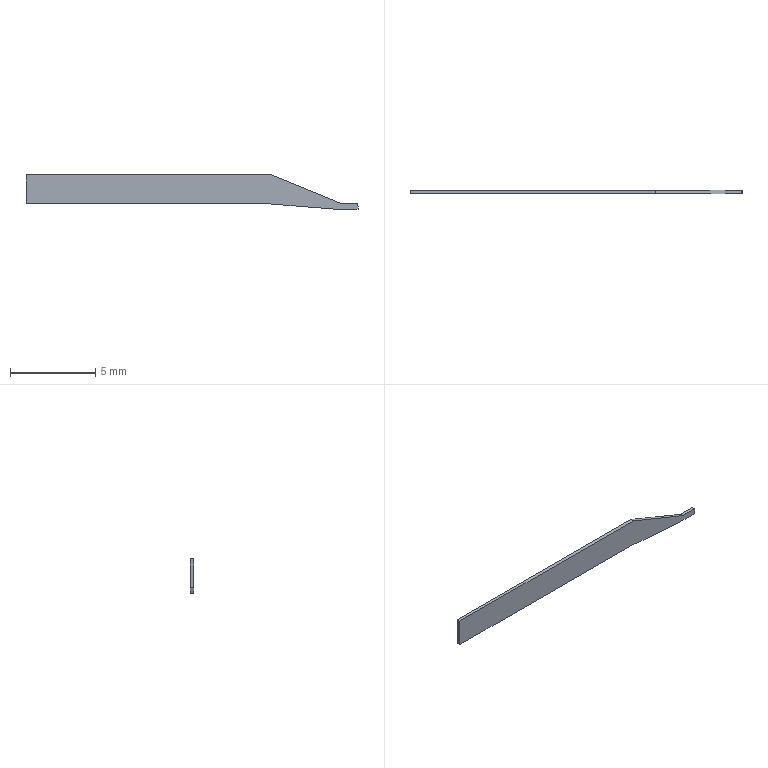Part | SolidWorks | features Extrusion 1 | 1 solid | 10 faces | box 19.5 x 0.2 x 2.02 mm | volume 5.825 mm3 | plane 10
STEP:
#1=CARTESIAN_POINT('',(0.,0.,-1.7));
#2=VERTEX_POINT('',#1);
#3=CARTESIAN_POINT('',(0.,0.,0.));
#4=VERTEX_POINT('',#3);
#5=CARTESIAN_POINT('',(0.,0.,0.));
#6=DIRECTION('',(0.,0.,1.));
#7=VECTOR('',#6,1000.);
#8=LINE('',#5,#7);
#9=EDGE_CURVE('',#2,#4,#8,.T.);
#10=ORIENTED_EDGE('',*,*,#9,.T.);
#11=CARTESIAN_POINT('',(0.,0.2,0.));
#12=VERTEX_POINT('',#11);
#13=CARTESIAN_POINT('',(0.,0.2,0.));
#14=DIRECTION('',(0.,-1.,0.));
#15=VECTOR('',#14,1000.);
#16=LINE('',#13,#15);
#17=EDGE_CURVE('',#12,#4,#16,.T.);
#18=ORIENTED_EDGE('',*,*,#17,.F.);
#19=CARTESIAN_POINT('',(0.,0.2,-1.7));
#20=VERTEX_POINT('',#19);
#21=CARTESIAN_POINT('',(0.,0.2,0.));
#22=DIRECTION('',(0.,0.,1.));
#23=VECTOR('',#22,1000.);
#24=LINE('',#21,#23);
#25=EDGE_CURVE('',#20,#12,#24,.T.);
#26=ORIENTED_EDGE('',*,*,#25,.F.);
#27=CARTESIAN_POINT('',(0.,0.2,-1.7));
#28=DIRECTION('',(0.,-1.,0.));
#29=VECTOR('',#28,1000.);
#30=LINE('',#27,#29);
#31=EDGE_CURVE('',#20,#2,#30,.T.);
#32=ORIENTED_EDGE('',*,*,#31,.T.);
#33=EDGE_LOOP('',(#10,#18,#26,#32));
#34=FACE_OUTER_BOUND('',#33,.T.);
#35=CARTESIAN_POINT('',(0.,0.2,0.));
#36=DIRECTION('',(1.,0.,0.));
#37=DIRECTION('',(0.,0.,-1.));
#38=AXIS2_PLACEMENT_3D('',#35,#36,#37);
#39=PLANE('',#38);
#40=ADVANCED_FACE('',(#34),#39,.F.);
#41=CARTESIAN_POINT('',(14.408,0.,0.));
#42=VERTEX_POINT('',#41);
#43=CARTESIAN_POINT('',(0.,0.,0.));
#44=DIRECTION('',(1.,0.,0.));
#45=VECTOR('',#44,1000.);
#46=LINE('',#43,#45);
#47=EDGE_CURVE('',#4,#42,#46,.T.);
#48=ORIENTED_EDGE('',*,*,#47,.T.);
#49=CARTESIAN_POINT('',(14.408,0.2,0.));
#50=VERTEX_POINT('',#49);
#51=CARTESIAN_POINT('',(14.408,0.2,0.));
#52=DIRECTION('',(0.,-1.,0.));
#53=VECTOR('',#52,1000.);
#54=LINE('',#51,#53);
#55=EDGE_CURVE('',#50,#42,#54,.T.);
#56=ORIENTED_EDGE('',*,*,#55,.F.);
#57=CARTESIAN_POINT('',(0.,0.2,0.));
#58=DIRECTION('',(1.,0.,0.));
#59=VECTOR('',#58,1000.);
#60=LINE('',#57,#59);
#61=EDGE_CURVE('',#12,#50,#60,.T.);
#62=ORIENTED_EDGE('',*,*,#61,.F.);
#63=ORIENTED_EDGE('',*,*,#17,.T.);
#64=EDGE_LOOP('',(#48,#56,#62,#63));
#65=FACE_OUTER_BOUND('',#64,.T.);
#66=CARTESIAN_POINT('',(0.,0.2,0.));
#67=DIRECTION('',(0.,0.,-1.));
#68=DIRECTION('',(-1.,0.,0.));
#69=AXIS2_PLACEMENT_3D('',#66,#67,#68);
#70=PLANE('',#69);
#71=ADVANCED_FACE('',(#65),#70,.F.);
#72=CARTESIAN_POINT('',(18.5,0.,-1.67));
#73=VERTEX_POINT('',#72);
#74=CARTESIAN_POINT('',(18.5,0.,-1.67));
#75=DIRECTION('',(0.9259,0.,-0.3778));
#76=VECTOR('',#75,1000.);
#77=LINE('',#74,#76);
#78=EDGE_CURVE('',#42,#73,#77,.T.);
#79=ORIENTED_EDGE('',*,*,#78,.T.);
#80=CARTESIAN_POINT('',(18.5,0.2,-1.67));
#81=VERTEX_POINT('',#80);
#82=CARTESIAN_POINT('',(18.5,0.2,-1.67));
#83=DIRECTION('',(0.,-1.,0.));
#84=VECTOR('',#83,1000.);
#85=LINE('',#82,#84);
#86=EDGE_CURVE('',#81,#73,#85,.T.);
#87=ORIENTED_EDGE('',*,*,#86,.F.);
#88=CARTESIAN_POINT('',(18.5,0.2,-1.67));
#89=DIRECTION('',(0.9259,0.,-0.3778));
#90=VECTOR('',#89,1000.);
#91=LINE('',#88,#90);
#92=EDGE_CURVE('',#50,#81,#91,.T.);
#93=ORIENTED_EDGE('',*,*,#92,.F.);
#94=ORIENTED_EDGE('',*,*,#55,.T.);
#95=EDGE_LOOP('',(#79,#87,#93,#94));
#96=FACE_OUTER_BOUND('',#95,.T.);
#97=CARTESIAN_POINT('',(18.5,0.2,-1.67));
#98=DIRECTION('',(-0.3778,0.,-0.9259));
#99=DIRECTION('',(-0.9259,0.,0.3778));
#100=AXIS2_PLACEMENT_3D('',#97,#98,#99);
#101=PLANE('',#100);
#102=ADVANCED_FACE('',(#96),#101,.F.);
#103=CARTESIAN_POINT('',(19.5,0.,-1.67));
#104=VERTEX_POINT('',#103);
#105=CARTESIAN_POINT('',(19.5,0.,-1.67));
#106=DIRECTION('',(1.,0.,0.));
#107=VECTOR('',#106,1000.);
#108=LINE('',#105,#107);
#109=EDGE_CURVE('',#73,#104,#108,.T.);
#110=ORIENTED_EDGE('',*,*,#109,.T.);
#111=CARTESIAN_POINT('',(19.5,0.2,-1.67));
#112=VERTEX_POINT('',#111);
#113=CARTESIAN_POINT('',(19.5,0.2,-1.67));
#114=DIRECTION('',(0.,-1.,0.));
#115=VECTOR('',#114,1000.);
#116=LINE('',#113,#115);
#117=EDGE_CURVE('',#112,#104,#116,.T.);
#118=ORIENTED_EDGE('',*,*,#117,.F.);
#119=CARTESIAN_POINT('',(19.5,0.2,-1.67));
#120=DIRECTION('',(1.,0.,0.));
#121=VECTOR('',#120,1000.);
#122=LINE('',#119,#121);
#123=EDGE_CURVE('',#81,#112,#122,.T.);
#124=ORIENTED_EDGE('',*,*,#123,.F.);
#125=ORIENTED_EDGE('',*,*,#86,.T.);
#126=EDGE_LOOP('',(#110,#118,#124,#125));
#127=FACE_OUTER_BOUND('',#126,.T.);
#128=CARTESIAN_POINT('',(19.5,0.2,-1.67));
#129=DIRECTION('',(0.,0.,-1.));
#130=DIRECTION('',(-1.,0.,0.));
#131=AXIS2_PLACEMENT_3D('',#128,#129,#130);
#132=PLANE('',#131);
#133=ADVANCED_FACE('',(#127),#132,.F.);
#134=CARTESIAN_POINT('',(19.5,0.,-2.02));
#135=VERTEX_POINT('',#134);
#136=CARTESIAN_POINT('',(19.5,0.,-1.67));
#137=DIRECTION('',(0.,0.,-1.));
#138=VECTOR('',#137,1000.);
#139=LINE('',#136,#138);
#140=EDGE_CURVE('',#104,#135,#139,.T.);
#141=ORIENTED_EDGE('',*,*,#140,.T.);
#142=CARTESIAN_POINT('',(19.5,0.2,-2.02));
#143=VERTEX_POINT('',#142);
#144=CARTESIAN_POINT('',(19.5,0.2,-2.02));
#145=DIRECTION('',(0.,-1.,0.));
#146=VECTOR('',#145,1000.);
#147=LINE('',#144,#146);
#148=EDGE_CURVE('',#143,#135,#147,.T.);
#149=ORIENTED_EDGE('',*,*,#148,.F.);
#150=CARTESIAN_POINT('',(19.5,0.2,-1.67));
#151=DIRECTION('',(0.,0.,-1.));
#152=VECTOR('',#151,1000.);
#153=LINE('',#150,#152);
#154=EDGE_CURVE('',#112,#143,#153,.T.);
#155=ORIENTED_EDGE('',*,*,#154,.F.);
#156=ORIENTED_EDGE('',*,*,#117,.T.);
#157=EDGE_LOOP('',(#141,#149,#155,#156));
#158=FACE_OUTER_BOUND('',#157,.T.);
#159=CARTESIAN_POINT('',(19.5,0.2,-1.67));
#160=DIRECTION('',(-1.,0.,0.));
#161=DIRECTION('',(0.,0.,1.));
#162=AXIS2_PLACEMENT_3D('',#159,#160,#161);
#163=PLANE('',#162);
#164=ADVANCED_FACE('',(#158),#163,.F.);
#165=CARTESIAN_POINT('',(18.177,0.,-2.02));
#166=VERTEX_POINT('',#165);
#167=CARTESIAN_POINT('',(18.177,0.,-2.02));
#168=DIRECTION('',(-1.,0.,0.));
#169=VECTOR('',#168,1000.);
#170=LINE('',#167,#169);
#171=EDGE_CURVE('',#135,#166,#170,.T.);
#172=ORIENTED_EDGE('',*,*,#171,.T.);
#173=CARTESIAN_POINT('',(18.177,0.2,-2.02));
#174=VERTEX_POINT('',#173);
#175=CARTESIAN_POINT('',(18.177,0.2,-2.02));
#176=DIRECTION('',(0.,-1.,0.));
#177=VECTOR('',#176,1000.);
#178=LINE('',#175,#177);
#179=EDGE_CURVE('',#174,#166,#178,.T.);
#180=ORIENTED_EDGE('',*,*,#179,.F.);
#181=CARTESIAN_POINT('',(18.177,0.2,-2.02));
#182=DIRECTION('',(-1.,0.,0.));
#183=VECTOR('',#182,1000.);
#184=LINE('',#181,#183);
#185=EDGE_CURVE('',#143,#174,#184,.T.);
#186=ORIENTED_EDGE('',*,*,#185,.F.);
#187=ORIENTED_EDGE('',*,*,#148,.T.);
#188=EDGE_LOOP('',(#172,#180,#186,#187));
#189=FACE_OUTER_BOUND('',#188,.T.);
#190=CARTESIAN_POINT('',(18.177,0.2,-2.02));
#191=DIRECTION('',(0.,0.,1.));
#192=DIRECTION('',(1.,0.,0.));
#193=AXIS2_PLACEMENT_3D('',#190,#191,#192);
#194=PLANE('',#193);
#195=ADVANCED_FACE('',(#189),#194,.F.);
#196=CARTESIAN_POINT('',(14.2,0.,-1.7));
#197=VERTEX_POINT('',#196);
#198=CARTESIAN_POINT('',(14.2,0.,-1.7));
#199=DIRECTION('',(-0.9968,0.,0.0802));
#200=VECTOR('',#199,1000.);
#201=LINE('',#198,#200);
#202=EDGE_CURVE('',#166,#197,#201,.T.);
#203=ORIENTED_EDGE('',*,*,#202,.T.);
#204=CARTESIAN_POINT('',(14.2,0.2,-1.7));
#205=VERTEX_POINT('',#204);
#206=CARTESIAN_POINT('',(14.2,0.2,-1.7));
#207=DIRECTION('',(0.,-1.,0.));
#208=VECTOR('',#207,1000.);
#209=LINE('',#206,#208);
#210=EDGE_CURVE('',#205,#197,#209,.T.);
#211=ORIENTED_EDGE('',*,*,#210,.F.);
#212=CARTESIAN_POINT('',(14.2,0.2,-1.7));
#213=DIRECTION('',(-0.9968,0.,0.0802));
#214=VECTOR('',#213,1000.);
#215=LINE('',#212,#214);
#216=EDGE_CURVE('',#174,#205,#215,.T.);
#217=ORIENTED_EDGE('',*,*,#216,.F.);
#218=ORIENTED_EDGE('',*,*,#179,.T.);
#219=EDGE_LOOP('',(#203,#211,#217,#218));
#220=FACE_OUTER_BOUND('',#219,.T.);
#221=CARTESIAN_POINT('',(14.2,0.2,-1.7));
#222=DIRECTION('',(0.0802,0.,0.9968));
#223=DIRECTION('',(0.9968,0.,-0.0802));
#224=AXIS2_PLACEMENT_3D('',#221,#222,#223);
#225=PLANE('',#224);
#226=ADVANCED_FACE('',(#220),#225,.F.);
#227=CARTESIAN_POINT('',(0.,0.,-1.7));
#228=DIRECTION('',(-1.,0.,0.));
#229=VECTOR('',#228,1000.);
#230=LINE('',#227,#229);
#231=EDGE_CURVE('',#197,#2,#230,.T.);
#232=ORIENTED_EDGE('',*,*,#231,.T.);
#233=ORIENTED_EDGE('',*,*,#31,.F.);
#234=CARTESIAN_POINT('',(0.,0.2,-1.7));
#235=DIRECTION('',(-1.,0.,0.));
#236=VECTOR('',#235,1000.);
#237=LINE('',#234,#236);
#238=EDGE_CURVE('',#205,#20,#237,.T.);
#239=ORIENTED_EDGE('',*,*,#238,.F.);
#240=ORIENTED_EDGE('',*,*,#210,.T.);
#241=EDGE_LOOP('',(#232,#233,#239,#240));
#242=FACE_OUTER_BOUND('',#241,.T.);
#243=CARTESIAN_POINT('',(0.,0.2,-1.7));
#244=DIRECTION('',(0.,0.,1.));
#245=DIRECTION('',(1.,0.,0.));
#246=AXIS2_PLACEMENT_3D('',#243,#244,#245);
#247=PLANE('',#246);
#248=ADVANCED_FACE('',(#242),#247,.F.);
#249=ORIENTED_EDGE('',*,*,#25,.T.);
#250=ORIENTED_EDGE('',*,*,#61,.T.);
#251=ORIENTED_EDGE('',*,*,#92,.T.);
#252=ORIENTED_EDGE('',*,*,#123,.T.);
#253=ORIENTED_EDGE('',*,*,#154,.T.);
#254=ORIENTED_EDGE('',*,*,#185,.T.);
#255=ORIENTED_EDGE('',*,*,#216,.T.);
#256=ORIENTED_EDGE('',*,*,#238,.T.);
#257=EDGE_LOOP('',(#249,#250,#251,#252,#253,#254,#255,#256));
#258=FACE_OUTER_BOUND('',#257,.T.);
#259=CARTESIAN_POINT('',(0.,0.2,0.));
#260=DIRECTION('',(0.,-1.,0.));
#261=DIRECTION('',(0.,0.,-1.));
#262=AXIS2_PLACEMENT_3D('',#259,#260,#261);
#263=PLANE('',#262);
#264=ADVANCED_FACE('',(#258),#263,.F.);
#265=ORIENTED_EDGE('',*,*,#9,.F.);
#266=ORIENTED_EDGE('',*,*,#231,.F.);
#267=ORIENTED_EDGE('',*,*,#202,.F.);
#268=ORIENTED_EDGE('',*,*,#171,.F.);
#269=ORIENTED_EDGE('',*,*,#140,.F.);
#270=ORIENTED_EDGE('',*,*,#109,.F.);
#271=ORIENTED_EDGE('',*,*,#78,.F.);
#272=ORIENTED_EDGE('',*,*,#47,.F.);
#273=EDGE_LOOP('',(#265,#266,#267,#268,#269,#270,#271,#272));
#274=FACE_OUTER_BOUND('',#273,.T.);
#275=CARTESIAN_POINT('',(0.,0.,0.));
#276=DIRECTION('',(0.,-1.,0.));
#277=DIRECTION('',(0.,0.,-1.));
#278=AXIS2_PLACEMENT_3D('',#275,#276,#277);
#279=PLANE('',#278);
#280=ADVANCED_FACE('',(#274),#279,.T.);
#281=CLOSED_SHELL('',(#40,#71,#102,#133,#164,#195,#226,#248,#264,#280));
#282=MANIFOLD_SOLID_BREP('',#281);
#283=CARTESIAN_POINT('',(0.,0.,0.));
#284=DIRECTION('',(0.,0.,1.));
#285=DIRECTION('',(1.,0.,0.));
#286=AXIS2_PLACEMENT_3D('',#283,#284,#285);
#287=(LENGTH_UNIT()NAMED_UNIT(*)SI_UNIT(.MILLI.,.METRE.));
#288=UNCERTAINTY_MEASURE_WITH_UNIT(LENGTH_MEASURE(0.00001),#287,'','');
#289=(NAMED_UNIT(*)PLANE_ANGLE_UNIT()SI_UNIT($,.RADIAN.));
#290=(NAMED_UNIT(*)SI_UNIT($,.STERADIAN.)SOLID_ANGLE_UNIT());
#291=(GEOMETRIC_REPRESENTATION_CONTEXT(3)GLOBAL_UNCERTAINTY_ASSIGNED_CONTEXT((#288))GLOBAL_UNIT_ASSIGNED_CONTEXT((#287,#289,#290))REPRESENTATION_CONTEXT('',''));
#292=ADVANCED_BREP_SHAPE_REPRESENTATION('',(#282,#286),#291);